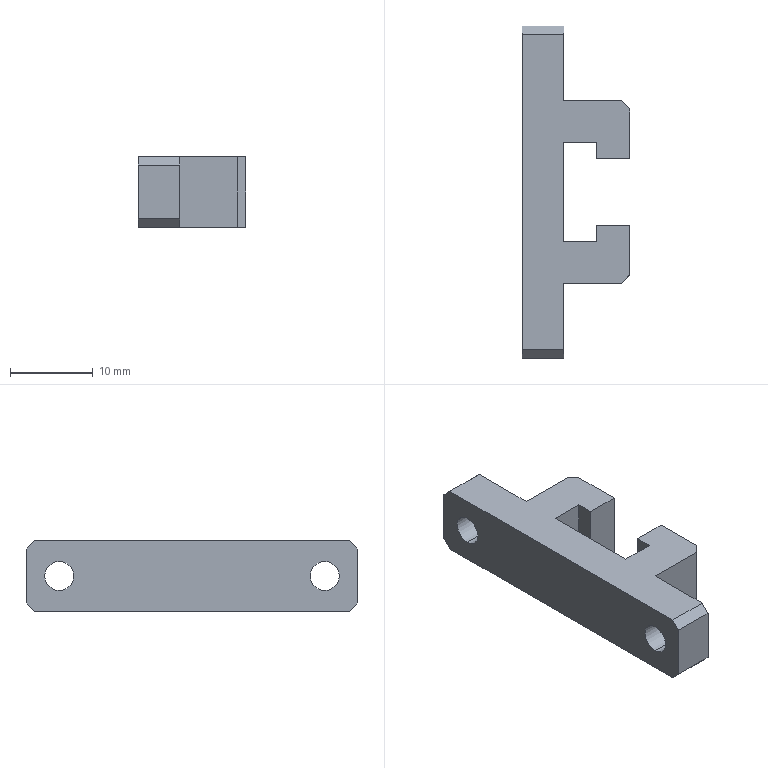Part | STEP file | lifting link plate | 1 solid | 28 faces | box 13 x 40 x 8.5 mm | volume 2401 mm3 | plane 24 | cylinder 4 | commonest cylinder face diameters 3.5 x4